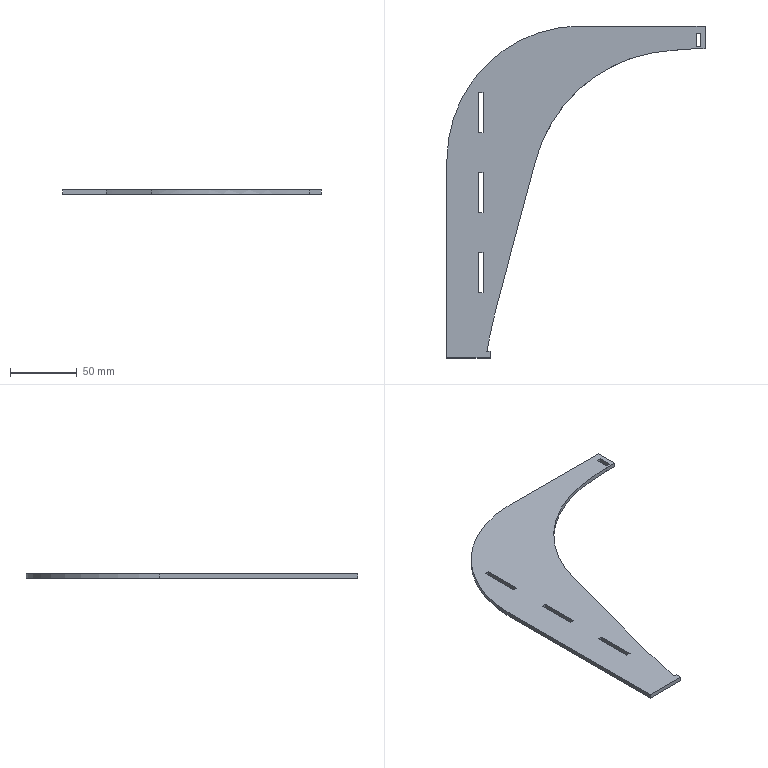Part | SolidWorks | features FlatPattern 1, SMBaseFlange 1, SheetMetal 1 | 1 solid | 31 faces | box 193.405 x 248.788 x 3.2 mm | volume 50560 mm3 | plane 26 | spline 3 | cylinder 2 | commonest cylinder face diameters 200 x1 887.053 x1
STEP:
#1=CARTESIAN_POINT('',(-170.654,-16.016,0.));
#2=VERTEX_POINT('',#1);
#3=CARTESIAN_POINT('',(-52.245,67.625,0.));
#4=VERTEX_POINT('',#3);
#5=CARTESIAN_POINT('',(-170.654,-16.016,0.));
#6=CARTESIAN_POINT('',(-168.965,-9.713,0.));
#7=CARTESIAN_POINT('',(-166.726,-3.585,0.));
#8=CARTESIAN_POINT('',(-161.155,8.306,0.));
#9=CARTESIAN_POINT('',(-157.878,13.952,0.));
#10=CARTESIAN_POINT('',(-150.345,24.639,0.));
#11=CARTESIAN_POINT('',(-146.124,29.625,0.));
#12=CARTESIAN_POINT('',(-139.114,36.565,0.));
#13=CARTESIAN_POINT('',(-135.476,39.865,0.));
#14=CARTESIAN_POINT('',(-130.997,43.416,0.));
#15=CARTESIAN_POINT('',(-129.027,44.874,0.));
#16=CARTESIAN_POINT('',(-127.703,45.832,0.));
#17=CARTESIAN_POINT('',(-127.037,46.303,0.));
#18=CARTESIAN_POINT('',(-120.965,50.494,0.));
#19=CARTESIAN_POINT('',(-115.278,53.719,0.));
#20=CARTESIAN_POINT('',(-103.335,59.164,0.));
#21=CARTESIAN_POINT('',(-97.175,61.342,0.));
#22=CARTESIAN_POINT('',(-89.232,63.383,0.));
#23=CARTESIAN_POINT('',(-86.84,63.941,0.));
#24=CARTESIAN_POINT('',(-84.034,64.499,0.));
#25=CARTESIAN_POINT('',(-82.627,64.754,0.));
#26=CARTESIAN_POINT('',(-82.023,64.858,0.));
#27=CARTESIAN_POINT('',(-81.62,64.926,0.));
#28=CARTESIAN_POINT('',(-81.417,64.96,0.));
#29=CARTESIAN_POINT('',(-80.419,65.124,0.));
#30=CARTESIAN_POINT('',(-79.214,65.308,0.));
#31=CARTESIAN_POINT('',(-77.793,65.502,0.));
#32=CARTESIAN_POINT('',(-77.079,65.593,0.));
#33=CARTESIAN_POINT('',(-76.721,65.637,0.));
#34=CARTESIAN_POINT('',(-76.542,65.659,0.));
#35=CARTESIAN_POINT('',(-76.452,65.67,0.));
#36=CARTESIAN_POINT('',(-76.407,65.676,0.));
#37=CARTESIAN_POINT('',(-76.388,65.678,0.));
#38=CARTESIAN_POINT('',(-76.375,65.679,0.));
#39=CARTESIAN_POINT('',(-76.368,65.68,0.));
#40=CARTESIAN_POINT('',(-75.713,65.759,0.));
#41=CARTESIAN_POINT('',(-74.62,65.88,0.));
#42=CARTESIAN_POINT('',(-73.139,66.029,0.));
#43=CARTESIAN_POINT('',(-72.346,66.106,0.));
#44=CARTESIAN_POINT('',(-71.937,66.145,0.));
#45=CARTESIAN_POINT('',(-71.729,66.164,0.));
#46=CARTESIAN_POINT('',(-71.625,66.174,0.));
#47=CARTESIAN_POINT('',(-71.572,66.179,0.));
#48=CARTESIAN_POINT('',(-71.55,66.181,0.));
#49=CARTESIAN_POINT('',(-71.535,66.182,0.));
#50=CARTESIAN_POINT('',(-71.526,66.183,0.));
#51=CARTESIAN_POINT('',(-65.156,66.776,0.));
#52=CARTESIAN_POINT('',(-58.732,67.256,0.));
#53=CARTESIAN_POINT('',(-52.245,67.625,0.));
#54=B_SPLINE_CURVE_WITH_KNOTS('',3,(#5,#6,#7,#8,#9,#10,#11,#12,#13,#14,#15,#16,#17,#18,#19,#20,#21,#22,#23,#24,#25,#26,#27,#28,#29,#30,#31,#32,#33,#34,#35,#36,#37,#38,#39,#40,#41,#42,#43,#44,#45,#46,#47,#48,#49,#50,#51,#52,#53),.UNSPECIFIED.,.F.,.F.,(4,2,2,2,1,1,2,2,2,2,1,1,1,2,2,1,1,1,1,1,1,1,2,2,1,1,1,1,1,1,1,2,2,4),(0.,0.125,0.25,0.375,0.4375,0.4688,0.4844,0.5,0.625,0.75,0.7813,0.7969,0.8047,0.8086,0.8125,0.8281,0.8359,0.8398,0.8418,0.8428,0.8433,0.8435,0.8436,0.8438,0.8594,0.8672,0.8711,0.873,0.874,0.8745,0.8748,0.8749,0.875,1.),.UNSPECIFIED.);
#55=EDGE_CURVE('',#2,#4,#54,.T.);
#56=ORIENTED_EDGE('',*,*,#55,.F.);
#57=CARTESIAN_POINT('',(-170.654,-16.016,-3.2));
#58=VERTEX_POINT('',#57);
#59=CARTESIAN_POINT('',(-170.654,-16.016,-3.2));
#60=DIRECTION('',(0.,0.,1.));
#61=VECTOR('',#60,1000.);
#62=LINE('',#59,#61);
#63=EDGE_CURVE('',#58,#2,#62,.T.);
#64=ORIENTED_EDGE('',*,*,#63,.F.);
#65=CARTESIAN_POINT('',(-52.245,67.625,-3.2));
#66=VERTEX_POINT('',#65);
#67=CARTESIAN_POINT('',(-170.654,-16.016,-3.2));
#68=CARTESIAN_POINT('',(-167.275,-3.408,-3.2));
#69=CARTESIAN_POINT('',(-161.645,8.608,-3.2));
#70=CARTESIAN_POINT('',(-146.578,29.983,-3.2));
#71=CARTESIAN_POINT('',(-137.134,39.334,-3.2));
#72=CARTESIAN_POINT('',(-120.976,50.486,-3.2));
#73=CARTESIAN_POINT('',(-115.261,53.727,-3.2));
#74=CARTESIAN_POINT('',(-103.352,59.157,-3.2));
#75=CARTESIAN_POINT('',(-97.158,61.346,-3.2));
#76=CARTESIAN_POINT('',(-87.652,63.789,-3.2));
#77=CARTESIAN_POINT('',(-84.447,64.463,-3.2));
#78=CARTESIAN_POINT('',(-79.602,65.258,-3.2));
#79=CARTESIAN_POINT('',(-77.981,65.487,-3.2));
#80=CARTESIAN_POINT('',(-74.744,65.875,-3.2));
#81=CARTESIAN_POINT('',(-73.129,66.034,-3.2));
#82=CARTESIAN_POINT('',(-68.301,66.483,-3.2));
#83=CARTESIAN_POINT('',(-65.1,66.748,-3.2));
#84=CARTESIAN_POINT('',(-58.675,67.229,-3.2));
#85=CARTESIAN_POINT('',(-55.46,67.442,-3.2));
#86=CARTESIAN_POINT('',(-52.245,67.625,-3.2));
#87=B_SPLINE_CURVE_WITH_KNOTS('',3,(#67,#68,#69,#70,#71,#72,#73,#74,#75,#76,#77,#78,#79,#80,#81,#82,#83,#84,#85,#86),.UNSPECIFIED.,.F.,.F.,(4,2,2,2,2,2,2,2,2,4),(0.,0.25,0.5,0.625,0.75,0.8125,0.8438,0.875,0.9375,1.),.UNSPECIFIED.);
#88=EDGE_CURVE('',#58,#66,#87,.T.);
#89=ORIENTED_EDGE('',*,*,#88,.T.);
#90=CARTESIAN_POINT('',(-52.245,67.625,-3.2));
#91=DIRECTION('',(0.,0.,1.));
#92=VECTOR('',#91,1000.);
#93=LINE('',#90,#92);
#94=EDGE_CURVE('',#66,#4,#93,.T.);
#95=ORIENTED_EDGE('',*,*,#94,.T.);
#96=EDGE_LOOP('',(#56,#64,#89,#95));
#97=FACE_OUTER_BOUND('',#96,.T.);
#98=CARTESIAN_POINT('',(-170.654,-16.016,-3.2));
#99=CARTESIAN_POINT('',(-170.654,-16.016,0.));
#100=CARTESIAN_POINT('',(-167.275,-3.408,-3.2));
#101=CARTESIAN_POINT('',(-167.275,-3.408,0.));
#102=CARTESIAN_POINT('',(-161.645,8.608,-3.2));
#103=CARTESIAN_POINT('',(-161.645,8.608,0.));
#104=CARTESIAN_POINT('',(-146.578,29.983,-3.2));
#105=CARTESIAN_POINT('',(-146.578,29.983,0.));
#106=CARTESIAN_POINT('',(-137.134,39.334,-3.2));
#107=CARTESIAN_POINT('',(-137.134,39.334,0.));
#108=CARTESIAN_POINT('',(-120.976,50.486,-3.2));
#109=CARTESIAN_POINT('',(-120.976,50.486,0.));
#110=CARTESIAN_POINT('',(-115.261,53.727,-3.2));
#111=CARTESIAN_POINT('',(-115.261,53.727,0.));
#112=CARTESIAN_POINT('',(-103.352,59.157,-3.2));
#113=CARTESIAN_POINT('',(-103.352,59.157,0.));
#114=CARTESIAN_POINT('',(-97.158,61.346,-3.2));
#115=CARTESIAN_POINT('',(-97.158,61.346,0.));
#116=CARTESIAN_POINT('',(-87.652,63.789,-3.2));
#117=CARTESIAN_POINT('',(-87.652,63.789,0.));
#118=CARTESIAN_POINT('',(-84.447,64.463,-3.2));
#119=CARTESIAN_POINT('',(-84.447,64.463,0.));
#120=CARTESIAN_POINT('',(-79.602,65.258,-3.2));
#121=CARTESIAN_POINT('',(-79.602,65.258,0.));
#122=CARTESIAN_POINT('',(-77.981,65.487,-3.2));
#123=CARTESIAN_POINT('',(-77.981,65.487,0.));
#124=CARTESIAN_POINT('',(-74.744,65.875,-3.2));
#125=CARTESIAN_POINT('',(-74.744,65.875,0.));
#126=CARTESIAN_POINT('',(-73.129,66.034,-3.2));
#127=CARTESIAN_POINT('',(-73.129,66.034,0.));
#128=CARTESIAN_POINT('',(-68.301,66.483,-3.2));
#129=CARTESIAN_POINT('',(-68.301,66.483,0.));
#130=CARTESIAN_POINT('',(-65.1,66.748,-3.2));
#131=CARTESIAN_POINT('',(-65.1,66.748,0.));
#132=CARTESIAN_POINT('',(-58.675,67.229,-3.2));
#133=CARTESIAN_POINT('',(-58.675,67.229,0.));
#134=CARTESIAN_POINT('',(-55.46,67.442,-3.2));
#135=CARTESIAN_POINT('',(-55.46,67.442,0.));
#136=CARTESIAN_POINT('',(-52.245,67.625,-3.2));
#137=CARTESIAN_POINT('',(-52.245,67.625,0.));
#138=B_SPLINE_SURFACE_WITH_KNOTS('',3,1,((#98,#99),(#100,#101),(#102,#103),(#104,#105),(#106,#107),(#108,#109),(#110,#111),(#112,#113),(#114,#115),(#116,#117),(#118,#119),(#120,#121),(#122,#123),(#124,#125),(#126,#127),(#128,#129),(#130,#131),(#132,#133),(#134,#135),(#136,#137)),.UNSPECIFIED.,.F.,.F.,.F.,(4,2,2,2,2,2,2,2,2,4),(2,2),(0.,0.25,0.5,0.625,0.75,0.8125,0.8438,0.875,0.9375,1.),(0.,1.),.UNSPECIFIED.);
#139=ADVANCED_FACE('',(#97),#138,.T.);
#140=CARTESIAN_POINT('',(-197.512,-116.241,0.));
#141=VERTEX_POINT('',#140);
#142=CARTESIAN_POINT('',(-170.654,-16.016,0.));
#143=DIRECTION('',(0.2588,0.9659,0.));
#144=VECTOR('',#143,1000.);
#145=LINE('',#142,#144);
#146=EDGE_CURVE('',#141,#2,#145,.T.);
#147=ORIENTED_EDGE('',*,*,#146,.F.);
#148=CARTESIAN_POINT('',(-197.512,-116.241,-3.2));
#149=VERTEX_POINT('',#148);
#150=CARTESIAN_POINT('',(-197.512,-116.241,-3.2));
#151=DIRECTION('',(0.,0.,1.));
#152=VECTOR('',#151,1000.);
#153=LINE('',#150,#152);
#154=EDGE_CURVE('',#149,#141,#153,.T.);
#155=ORIENTED_EDGE('',*,*,#154,.F.);
#156=CARTESIAN_POINT('',(-170.654,-16.016,-3.2));
#157=DIRECTION('',(0.2588,0.9659,0.));
#158=VECTOR('',#157,1000.);
#159=LINE('',#156,#158);
#160=EDGE_CURVE('',#149,#58,#159,.T.);
#161=ORIENTED_EDGE('',*,*,#160,.T.);
#162=ORIENTED_EDGE('',*,*,#63,.T.);
#163=EDGE_LOOP('',(#147,#155,#161,#162));
#164=FACE_OUTER_BOUND('',#163,.T.);
#165=CARTESIAN_POINT('',(-170.654,-16.016,-3.2));
#166=DIRECTION('',(0.9659,-0.2588,0.));
#167=DIRECTION('',(0.2588,0.9659,0.));
#168=AXIS2_PLACEMENT_3D('',#165,#166,#167);
#169=PLANE('',#168);
#170=ADVANCED_FACE('',(#164),#169,.T.);
#171=CARTESIAN_POINT('',(-204.762,-146.756,0.));
#172=VERTEX_POINT('',#171);
#173=CARTESIAN_POINT('',(230.108,-233.959,0.));
#174=DIRECTION('',(0.,0.,-1.));
#175=DIRECTION('',(-1.,0.,0.));
#176=AXIS2_PLACEMENT_3D('',#173,#174,#175);
#177=CIRCLE('',#176,443.526);
#178=EDGE_CURVE('',#172,#141,#177,.T.);
#179=ORIENTED_EDGE('',*,*,#178,.F.);
#180=CARTESIAN_POINT('',(-204.762,-146.756,-3.2));
#181=VERTEX_POINT('',#180);
#182=CARTESIAN_POINT('',(-204.762,-146.756,-3.2));
#183=DIRECTION('',(0.,0.,1.));
#184=VECTOR('',#183,1000.);
#185=LINE('',#182,#184);
#186=EDGE_CURVE('',#181,#172,#185,.T.);
#187=ORIENTED_EDGE('',*,*,#186,.F.);
#188=CARTESIAN_POINT('',(230.108,-233.959,-3.2));
#189=DIRECTION('',(0.,0.,-1.));
#190=DIRECTION('',(-1.,0.,0.));
#191=AXIS2_PLACEMENT_3D('',#188,#189,#190);
#192=CIRCLE('',#191,443.526);
#193=EDGE_CURVE('',#181,#149,#192,.T.);
#194=ORIENTED_EDGE('',*,*,#193,.T.);
#195=ORIENTED_EDGE('',*,*,#154,.T.);
#196=EDGE_LOOP('',(#179,#187,#194,#195));
#197=FACE_OUTER_BOUND('',#196,.T.);
#198=CARTESIAN_POINT('',(230.108,-233.959,-3.2));
#199=DIRECTION('',(0.,0.,1.));
#200=DIRECTION('',(1.,0.,0.));
#201=AXIS2_PLACEMENT_3D('',#198,#199,#200);
#202=CYLINDRICAL_SURFACE('',#201,443.526);
#203=ADVANCED_FACE('',(#197),#202,.F.);
#204=CARTESIAN_POINT('',(-207.067,-158.321,0.));
#205=VERTEX_POINT('',#204);
#206=CARTESIAN_POINT('',(-207.067,-158.321,0.));
#207=CARTESIAN_POINT('',(-206.479,-155.308,0.));
#208=CARTESIAN_POINT('',(-205.71,-151.453,0.));
#209=CARTESIAN_POINT('',(-204.762,-146.756,0.));
#210=B_SPLINE_CURVE_WITH_KNOTS('',3,(#206,#207,#208,#209),.UNSPECIFIED.,.F.,.F.,(4,4),(0.,1.),.UNSPECIFIED.);
#211=EDGE_CURVE('',#205,#172,#210,.T.);
#212=ORIENTED_EDGE('',*,*,#211,.F.);
#213=CARTESIAN_POINT('',(-207.067,-158.321,-3.2));
#214=VERTEX_POINT('',#213);
#215=CARTESIAN_POINT('',(-207.067,-158.321,-3.2));
#216=DIRECTION('',(0.,0.,1.));
#217=VECTOR('',#216,1000.);
#218=LINE('',#215,#217);
#219=EDGE_CURVE('',#214,#205,#218,.T.);
#220=ORIENTED_EDGE('',*,*,#219,.F.);
#221=CARTESIAN_POINT('',(-207.067,-158.321,-3.2));
#222=CARTESIAN_POINT('',(-206.57,-155.776,-3.2));
#223=CARTESIAN_POINT('',(-205.994,-152.886,-3.2));
#224=CARTESIAN_POINT('',(-205.529,-150.554,-3.2));
#225=CARTESIAN_POINT('',(-204.762,-146.756,-3.2));
#226=B_SPLINE_CURVE_WITH_KNOTS('',2,(#221,#222,#223,#224,#225),.UNSPECIFIED.,.F.,.F.,(3,2,3),(0.,0.5,1.),.UNSPECIFIED.);
#227=EDGE_CURVE('',#214,#181,#226,.T.);
#228=ORIENTED_EDGE('',*,*,#227,.T.);
#229=ORIENTED_EDGE('',*,*,#186,.T.);
#230=EDGE_LOOP('',(#212,#220,#228,#229));
#231=FACE_OUTER_BOUND('',#230,.T.);
#232=CARTESIAN_POINT('',(-207.067,-158.321,-3.2));
#233=CARTESIAN_POINT('',(-207.067,-158.321,0.));
#234=CARTESIAN_POINT('',(-206.57,-155.776,-3.2));
#235=CARTESIAN_POINT('',(-206.57,-155.776,0.));
#236=CARTESIAN_POINT('',(-205.994,-152.886,-3.2));
#237=CARTESIAN_POINT('',(-205.994,-152.886,0.));
#238=CARTESIAN_POINT('',(-205.529,-150.554,-3.2));
#239=CARTESIAN_POINT('',(-205.529,-150.554,0.));
#240=CARTESIAN_POINT('',(-204.762,-146.756,-3.2));
#241=CARTESIAN_POINT('',(-204.762,-146.756,0.));
#242=B_SPLINE_SURFACE_WITH_KNOTS('',2,1,((#232,#233),(#234,#235),(#236,#237),(#238,#239),(#240,#241)),.UNSPECIFIED.,.F.,.F.,.F.,(3,2,3),(2,2),(0.,0.5,1.),(0.,1.),.UNSPECIFIED.);
#243=ADVANCED_FACE('',(#231),#242,.T.);
#244=CARTESIAN_POINT('',(-207.184,-159.22,0.));
#245=VERTEX_POINT('',#244);
#246=CARTESIAN_POINT('',(-207.184,-159.22,0.));
#247=CARTESIAN_POINT('',(-207.159,-158.917,0.));
#248=CARTESIAN_POINT('',(-207.12,-158.617,0.));
#249=CARTESIAN_POINT('',(-207.067,-158.321,0.));
#250=B_SPLINE_CURVE_WITH_KNOTS('',3,(#246,#247,#248,#249),.UNSPECIFIED.,.F.,.F.,(4,4),(0.,1.),.UNSPECIFIED.);
#251=EDGE_CURVE('',#245,#205,#250,.T.);
#252=ORIENTED_EDGE('',*,*,#251,.F.);
#253=CARTESIAN_POINT('',(-207.184,-159.22,-3.2));
#254=VERTEX_POINT('',#253);
#255=CARTESIAN_POINT('',(-207.184,-159.22,-3.2));
#256=DIRECTION('',(0.,0.,1.));
#257=VECTOR('',#256,1000.);
#258=LINE('',#255,#257);
#259=EDGE_CURVE('',#254,#245,#258,.T.);
#260=ORIENTED_EDGE('',*,*,#259,.F.);
#261=CARTESIAN_POINT('',(-207.184,-159.22,-3.2));
#262=CARTESIAN_POINT('',(-207.172,-159.069,-3.2));
#263=CARTESIAN_POINT('',(-207.146,-158.766,-3.2));
#264=CARTESIAN_POINT('',(-207.094,-158.469,-3.2));
#265=CARTESIAN_POINT('',(-207.067,-158.321,-3.2));
#266=B_SPLINE_CURVE_WITH_KNOTS('',3,(#261,#262,#263,#264,#265),.UNSPECIFIED.,.F.,.F.,(4,1,4),(0.,0.5005,1.),.UNSPECIFIED.);
#267=EDGE_CURVE('',#254,#214,#266,.T.);
#268=ORIENTED_EDGE('',*,*,#267,.T.);
#269=ORIENTED_EDGE('',*,*,#219,.T.);
#270=EDGE_LOOP('',(#252,#260,#268,#269));
#271=FACE_OUTER_BOUND('',#270,.T.);
#272=CARTESIAN_POINT('',(-207.184,-159.22,-3.2));
#273=CARTESIAN_POINT('',(-207.184,-159.22,0.));
#274=CARTESIAN_POINT('',(-207.172,-159.069,-3.2));
#275=CARTESIAN_POINT('',(-207.172,-159.069,0.));
#276=CARTESIAN_POINT('',(-207.146,-158.766,-3.2));
#277=CARTESIAN_POINT('',(-207.146,-158.766,0.));
#278=CARTESIAN_POINT('',(-207.094,-158.469,-3.2));
#279=CARTESIAN_POINT('',(-207.094,-158.469,0.));
#280=CARTESIAN_POINT('',(-207.067,-158.321,-3.2));
#281=CARTESIAN_POINT('',(-207.067,-158.321,0.));
#282=B_SPLINE_SURFACE_WITH_KNOTS('',3,1,((#272,#273),(#274,#275),(#276,#277),(#278,#279),(#280,#281)),.UNSPECIFIED.,.F.,.F.,.F.,(4,1,4),(2,2),(0.,0.5005,1.),(0.,1.),.UNSPECIFIED.);
#283=ADVANCED_FACE('',(#271),#282,.T.);
#284=CARTESIAN_POINT('',(-204.879,-159.063,0.));
#285=VERTEX_POINT('',#284);
#286=CARTESIAN_POINT('',(-207.184,-159.22,0.));
#287=DIRECTION('',(-0.9977,-0.06788,0.));
#288=VECTOR('',#287,1000.);
#289=LINE('',#286,#288);
#290=EDGE_CURVE('',#285,#245,#289,.T.);
#291=ORIENTED_EDGE('',*,*,#290,.F.);
#292=CARTESIAN_POINT('',(-204.879,-159.063,-3.2));
#293=VERTEX_POINT('',#292);
#294=CARTESIAN_POINT('',(-204.879,-159.063,-3.2));
#295=DIRECTION('',(0.,0.,1.));
#296=VECTOR('',#295,1000.);
#297=LINE('',#294,#296);
#298=EDGE_CURVE('',#293,#285,#297,.T.);
#299=ORIENTED_EDGE('',*,*,#298,.F.);
#300=CARTESIAN_POINT('',(-207.184,-159.22,-3.2));
#301=DIRECTION('',(-0.9977,-0.06788,0.));
#302=VECTOR('',#301,1000.);
#303=LINE('',#300,#302);
#304=EDGE_CURVE('',#293,#254,#303,.T.);
#305=ORIENTED_EDGE('',*,*,#304,.T.);
#306=ORIENTED_EDGE('',*,*,#259,.T.);
#307=EDGE_LOOP('',(#291,#299,#305,#306));
#308=FACE_OUTER_BOUND('',#307,.T.);
#309=CARTESIAN_POINT('',(-207.184,-159.22,-3.2));
#310=DIRECTION('',(-0.06788,0.9977,0.));
#311=DIRECTION('',(-0.9977,-0.06788,0.));
#312=AXIS2_PLACEMENT_3D('',#309,#310,#311);
#313=PLANE('',#312);
#314=ADVANCED_FACE('',(#308),#313,.T.);
#315=CARTESIAN_POINT('',(-204.879,-164.063,0.));
#316=VERTEX_POINT('',#315);
#317=CARTESIAN_POINT('',(-204.879,-164.063,0.));
#318=DIRECTION('',(0.,1.,0.));
#319=VECTOR('',#318,1000.);
#320=LINE('',#317,#319);
#321=EDGE_CURVE('',#316,#285,#320,.T.);
#322=ORIENTED_EDGE('',*,*,#321,.F.);
#323=CARTESIAN_POINT('',(-204.879,-164.063,-3.2));
#324=VERTEX_POINT('',#323);
#325=CARTESIAN_POINT('',(-204.879,-164.063,-3.2));
#326=DIRECTION('',(0.,0.,1.));
#327=VECTOR('',#326,1000.);
#328=LINE('',#325,#327);
#329=EDGE_CURVE('',#324,#316,#328,.T.);
#330=ORIENTED_EDGE('',*,*,#329,.F.);
#331=CARTESIAN_POINT('',(-204.879,-164.063,-3.2));
#332=DIRECTION('',(0.,1.,0.));
#333=VECTOR('',#332,1000.);
#334=LINE('',#331,#333);
#335=EDGE_CURVE('',#324,#293,#334,.T.);
#336=ORIENTED_EDGE('',*,*,#335,.T.);
#337=ORIENTED_EDGE('',*,*,#298,.T.);
#338=EDGE_LOOP('',(#322,#330,#336,#337));
#339=FACE_OUTER_BOUND('',#338,.T.);
#340=CARTESIAN_POINT('',(-204.879,-164.063,-3.2));
#341=DIRECTION('',(1.,0.,0.));
#342=DIRECTION('',(0.,1.,0.));
#343=AXIS2_PLACEMENT_3D('',#340,#341,#342);
#344=PLANE('',#343);
#345=ADVANCED_FACE('',(#339),#344,.T.);
#346=CARTESIAN_POINT('',(-237.15,-164.063,0.));
#347=VERTEX_POINT('',#346);
#348=CARTESIAN_POINT('',(-237.15,-164.063,0.));
#349=DIRECTION('',(1.,0.,0.));
#350=VECTOR('',#349,1000.);
#351=LINE('',#348,#350);
#352=EDGE_CURVE('',#347,#316,#351,.T.);
#353=ORIENTED_EDGE('',*,*,#352,.F.);
#354=CARTESIAN_POINT('',(-237.15,-164.063,-3.2));
#355=VERTEX_POINT('',#354);
#356=CARTESIAN_POINT('',(-237.15,-164.063,-3.2));
#357=DIRECTION('',(0.,0.,1.));
#358=VECTOR('',#357,1000.);
#359=LINE('',#356,#358);
#360=EDGE_CURVE('',#355,#347,#359,.T.);
#361=ORIENTED_EDGE('',*,*,#360,.F.);
#362=CARTESIAN_POINT('',(-237.15,-164.063,-3.2));
#363=DIRECTION('',(1.,0.,0.));
#364=VECTOR('',#363,1000.);
#365=LINE('',#362,#364);
#366=EDGE_CURVE('',#355,#324,#365,.T.);
#367=ORIENTED_EDGE('',*,*,#366,.T.);
#368=ORIENTED_EDGE('',*,*,#329,.T.);
#369=EDGE_LOOP('',(#353,#361,#367,#368));
#370=FACE_OUTER_BOUND('',#369,.T.);
#371=CARTESIAN_POINT('',(-237.15,-164.063,-3.2));
#372=DIRECTION('',(0.,-1.,0.));
#373=DIRECTION('',(0.,0.,-1.));
#374=AXIS2_PLACEMENT_3D('',#371,#372,#373);
#375=PLANE('',#374);
#376=ADVANCED_FACE('',(#370),#375,.T.);
#377=CARTESIAN_POINT('',(-237.15,-15.276,0.));
#378=VERTEX_POINT('',#377);
#379=CARTESIAN_POINT('',(-237.15,-15.276,0.));
#380=DIRECTION('',(0.,-1.,0.));
#381=VECTOR('',#380,1000.);
#382=LINE('',#379,#381);
#383=EDGE_CURVE('',#378,#347,#382,.T.);
#384=ORIENTED_EDGE('',*,*,#383,.F.);
#385=CARTESIAN_POINT('',(-237.15,-15.276,-3.2));
#386=VERTEX_POINT('',#385);
#387=CARTESIAN_POINT('',(-237.15,-15.276,-3.2));
#388=DIRECTION('',(0.,0.,1.));
#389=VECTOR('',#388,1000.);
#390=LINE('',#387,#389);
#391=EDGE_CURVE('',#386,#378,#390,.T.);
#392=ORIENTED_EDGE('',*,*,#391,.F.);
#393=CARTESIAN_POINT('',(-237.15,-15.276,-3.2));
#394=DIRECTION('',(0.,-1.,0.));
#395=VECTOR('',#394,1000.);
#396=LINE('',#393,#395);
#397=EDGE_CURVE('',#386,#355,#396,.T.);
#398=ORIENTED_EDGE('',*,*,#397,.T.);
#399=ORIENTED_EDGE('',*,*,#360,.T.);
#400=EDGE_LOOP('',(#384,#392,#398,#399));
#401=FACE_OUTER_BOUND('',#400,.T.);
#402=CARTESIAN_POINT('',(-237.15,-15.276,-3.2));
#403=DIRECTION('',(-1.,0.,0.));
#404=DIRECTION('',(0.,-1.,0.));
#405=AXIS2_PLACEMENT_3D('',#402,#403,#404);
#406=PLANE('',#405);
#407=ADVANCED_FACE('',(#401),#406,.T.);
#408=CARTESIAN_POINT('',(-137.15,84.724,0.));
#409=VERTEX_POINT('',#408);
#410=CARTESIAN_POINT('',(-137.15,-15.276,0.));
#411=DIRECTION('',(0.,0.,1.));
#412=DIRECTION('',(-1.,0.,0.));
#413=AXIS2_PLACEMENT_3D('',#410,#411,#412);
#414=CIRCLE('',#413,100.);
#415=EDGE_CURVE('',#409,#378,#414,.T.);
#416=ORIENTED_EDGE('',*,*,#415,.F.);
#417=CARTESIAN_POINT('',(-137.15,84.724,-3.2));
#418=VERTEX_POINT('',#417);
#419=CARTESIAN_POINT('',(-137.15,84.724,-3.2));
#420=DIRECTION('',(0.,0.,1.));
#421=VECTOR('',#420,1000.);
#422=LINE('',#419,#421);
#423=EDGE_CURVE('',#418,#409,#422,.T.);
#424=ORIENTED_EDGE('',*,*,#423,.F.);
#425=CARTESIAN_POINT('',(-137.15,-15.276,-3.2));
#426=DIRECTION('',(0.,0.,1.));
#427=DIRECTION('',(-1.,0.,0.));
#428=AXIS2_PLACEMENT_3D('',#425,#426,#427);
#429=CIRCLE('',#428,100.);
#430=EDGE_CURVE('',#418,#386,#429,.T.);
#431=ORIENTED_EDGE('',*,*,#430,.T.);
#432=ORIENTED_EDGE('',*,*,#391,.T.);
#433=EDGE_LOOP('',(#416,#424,#431,#432));
#434=FACE_OUTER_BOUND('',#433,.T.);
#435=CARTESIAN_POINT('',(-137.15,-15.276,-3.2));
#436=DIRECTION('',(0.,0.,1.));
#437=DIRECTION('',(1.,0.,0.));
#438=AXIS2_PLACEMENT_3D('',#435,#436,#437);
#439=CYLINDRICAL_SURFACE('',#438,100.);
#440=ADVANCED_FACE('',(#434),#439,.T.);
#441=CARTESIAN_POINT('',(-43.745,84.724,0.));
#442=VERTEX_POINT('',#441);
#443=CARTESIAN_POINT('',(-43.745,84.724,0.));
#444=DIRECTION('',(-1.,0.,0.));
#445=VECTOR('',#444,1000.);
#446=LINE('',#443,#445);
#447=EDGE_CURVE('',#442,#409,#446,.T.);
#448=ORIENTED_EDGE('',*,*,#447,.F.);
#449=CARTESIAN_POINT('',(-43.745,84.724,-3.2));
#450=VERTEX_POINT('',#449);
#451=CARTESIAN_POINT('',(-43.745,84.724,-3.2));
#452=DIRECTION('',(0.,0.,1.));
#453=VECTOR('',#452,1000.);
#454=LINE('',#451,#453);
#455=EDGE_CURVE('',#450,#442,#454,.T.);
#456=ORIENTED_EDGE('',*,*,#455,.F.);
#457=CARTESIAN_POINT('',(-43.745,84.724,-3.2));
#458=DIRECTION('',(-1.,0.,0.));
#459=VECTOR('',#458,1000.);
#460=LINE('',#457,#459);
#461=EDGE_CURVE('',#450,#418,#460,.T.);
#462=ORIENTED_EDGE('',*,*,#461,.T.);
#463=ORIENTED_EDGE('',*,*,#423,.T.);
#464=EDGE_LOOP('',(#448,#456,#462,#463));
#465=FACE_OUTER_BOUND('',#464,.T.);
#466=CARTESIAN_POINT('',(-43.745,84.724,-3.2));
#467=DIRECTION('',(0.,1.,0.));
#468=DIRECTION('',(-1.,0.,0.));
#469=AXIS2_PLACEMENT_3D('',#466,#467,#468);
#470=PLANE('',#469);
#471=ADVANCED_FACE('',(#465),#470,.T.);
#472=CARTESIAN_POINT('',(-43.745,67.625,0.));
#473=VERTEX_POINT('',#472);
#474=CARTESIAN_POINT('',(-43.745,84.724,0.));
#475=DIRECTION('',(0.,1.,0.));
#476=VECTOR('',#475,1000.);
#477=LINE('',#474,#476);
#478=EDGE_CURVE('',#473,#442,#477,.T.);
#479=ORIENTED_EDGE('',*,*,#478,.F.);
#480=CARTESIAN_POINT('',(-43.745,67.625,-3.2));
#481=VERTEX_POINT('',#480);
#482=CARTESIAN_POINT('',(-43.745,67.625,-3.2));
#483=DIRECTION('',(0.,0.,1.));
#484=VECTOR('',#483,1000.);
#485=LINE('',#482,#484);
#486=EDGE_CURVE('',#481,#473,#485,.T.);
#487=ORIENTED_EDGE('',*,*,#486,.F.);
#488=CARTESIAN_POINT('',(-43.745,84.724,-3.2));
#489=DIRECTION('',(0.,1.,0.));
#490=VECTOR('',#489,1000.);
#491=LINE('',#488,#490);
#492=EDGE_CURVE('',#481,#450,#491,.T.);
#493=ORIENTED_EDGE('',*,*,#492,.T.);
#494=ORIENTED_EDGE('',*,*,#455,.T.);
#495=EDGE_LOOP('',(#479,#487,#493,#494));
#496=FACE_OUTER_BOUND('',#495,.T.);
#497=CARTESIAN_POINT('',(-43.745,84.724,-3.2));
#498=DIRECTION('',(1.,0.,0.));
#499=DIRECTION('',(0.,0.,-1.));
#500=AXIS2_PLACEMENT_3D('',#497,#498,#499);
#501=PLANE('',#500);
#502=ADVANCED_FACE('',(#496),#501,.T.);
#503=CARTESIAN_POINT('',(-43.745,67.625,0.));
#504=DIRECTION('',(1.,0.,0.));
#505=VECTOR('',#504,1000.);
#506=LINE('',#503,#505);
#507=EDGE_CURVE('',#4,#473,#506,.T.);
#508=ORIENTED_EDGE('',*,*,#507,.F.);
#509=ORIENTED_EDGE('',*,*,#94,.F.);
#510=CARTESIAN_POINT('',(-43.745,67.625,-3.2));
#511=DIRECTION('',(1.,0.,0.));
#512=VECTOR('',#511,1000.);
#513=LINE('',#510,#512);
#514=EDGE_CURVE('',#66,#481,#513,.T.);
#515=ORIENTED_EDGE('',*,*,#514,.T.);
#516=ORIENTED_EDGE('',*,*,#486,.T.);
#517=EDGE_LOOP('',(#508,#509,#515,#516));
#518=FACE_OUTER_BOUND('',#517,.T.);
#519=CARTESIAN_POINT('',(-43.745,67.625,-3.2));
#520=DIRECTION('',(0.,-1.,0.));
#521=DIRECTION('',(0.,0.,-1.));
#522=AXIS2_PLACEMENT_3D('',#519,#520,#521);
#523=PLANE('',#522);
#524=ADVANCED_FACE('',(#518),#523,.T.);
#525=CARTESIAN_POINT('',(-213.292,-85.276,-3.2));
#526=VERTEX_POINT('',#525);
#527=CARTESIAN_POINT('',(-213.292,-115.276,-3.2));
#528=VERTEX_POINT('',#527);
#529=CARTESIAN_POINT('',(-213.292,-85.276,-3.2));
#530=DIRECTION('',(0.,-1.,0.));
#531=VECTOR('',#530,1000.);
#532=LINE('',#529,#531);
#533=EDGE_CURVE('',#526,#528,#532,.T.);
#534=ORIENTED_EDGE('',*,*,#533,.T.);
#535=CARTESIAN_POINT('',(-210.092,-115.276,-3.2));
#536=VERTEX_POINT('',#535);
#537=CARTESIAN_POINT('',(-213.292,-115.276,-3.2));
#538=DIRECTION('',(1.,0.,0.));
#539=VECTOR('',#538,1000.);
#540=LINE('',#537,#539);
#541=EDGE_CURVE('',#528,#536,#540,.T.);
#542=ORIENTED_EDGE('',*,*,#541,.T.);
#543=CARTESIAN_POINT('',(-210.092,-85.276,-3.2));
#544=VERTEX_POINT('',#543);
#545=CARTESIAN_POINT('',(-210.092,-85.276,-3.2));
#546=DIRECTION('',(0.,1.,0.));
#547=VECTOR('',#546,1000.);
#548=LINE('',#545,#547);
#549=EDGE_CURVE('',#536,#544,#548,.T.);
#550=ORIENTED_EDGE('',*,*,#549,.T.);
#551=CARTESIAN_POINT('',(-213.292,-85.276,-3.2));
#552=DIRECTION('',(-1.,0.,0.));
#553=VECTOR('',#552,1000.);
#554=LINE('',#551,#553);
#555=EDGE_CURVE('',#544,#526,#554,.T.);
#556=ORIENTED_EDGE('',*,*,#555,.T.);
#557=EDGE_LOOP('',(#534,#542,#550,#556));
#558=FACE_BOUND('',#557,.T.);
#559=CARTESIAN_POINT('',(-213.292,-25.276,-3.2));
#560=VERTEX_POINT('',#559);
#561=CARTESIAN_POINT('',(-213.292,-55.276,-3.2));
#562=VERTEX_POINT('',#561);
#563=CARTESIAN_POINT('',(-213.292,-25.276,-3.2));
#564=DIRECTION('',(0.,-1.,0.));
#565=VECTOR('',#564,1000.);
#566=LINE('',#563,#565);
#567=EDGE_CURVE('',#560,#562,#566,.T.);
#568=ORIENTED_EDGE('',*,*,#567,.T.);
#569=CARTESIAN_POINT('',(-210.092,-55.276,-3.2));
#570=VERTEX_POINT('',#569);
#571=CARTESIAN_POINT('',(-213.292,-55.276,-3.2));
#572=DIRECTION('',(1.,0.,0.));
#573=VECTOR('',#572,1000.);
#574=LINE('',#571,#573);
#575=EDGE_CURVE('',#562,#570,#574,.T.);
#576=ORIENTED_EDGE('',*,*,#575,.T.);
#577=CARTESIAN_POINT('',(-210.092,-25.276,-3.2));
#578=VERTEX_POINT('',#577);
#579=CARTESIAN_POINT('',(-210.092,-25.276,-3.2));
#580=DIRECTION('',(0.,1.,0.));
#581=VECTOR('',#580,1000.);
#582=LINE('',#579,#581);
#583=EDGE_CURVE('',#570,#578,#582,.T.);
#584=ORIENTED_EDGE('',*,*,#583,.T.);
#585=CARTESIAN_POINT('',(-213.292,-25.276,-3.2));
#586=DIRECTION('',(-1.,0.,0.));
#587=VECTOR('',#586,1000.);
#588=LINE('',#585,#587);
#589=EDGE_CURVE('',#578,#560,#588,.T.);
#590=ORIENTED_EDGE('',*,*,#589,.T.);
#591=EDGE_LOOP('',(#568,#576,#584,#590));
#592=FACE_BOUND('',#591,.T.);
#593=CARTESIAN_POINT('',(-213.292,34.724,-3.2));
#594=VERTEX_POINT('',#593);
#595=CARTESIAN_POINT('',(-213.292,4.724,-3.2));
#596=VERTEX_POINT('',#595);
#597=CARTESIAN_POINT('',(-213.292,34.724,-3.2));
#598=DIRECTION('',(0.,-1.,0.));
#599=VECTOR('',#598,1000.);
#600=LINE('',#597,#599);
#601=EDGE_CURVE('',#594,#596,#600,.T.);
#602=ORIENTED_EDGE('',*,*,#601,.T.);
#603=CARTESIAN_POINT('',(-210.092,4.724,-3.2));
#604=VERTEX_POINT('',#603);
#605=CARTESIAN_POINT('',(-213.292,4.724,-3.2));
#606=DIRECTION('',(1.,0.,0.));
#607=VECTOR('',#606,1000.);
#608=LINE('',#605,#607);
#609=EDGE_CURVE('',#596,#604,#608,.T.);
#610=ORIENTED_EDGE('',*,*,#609,.T.);
#611=CARTESIAN_POINT('',(-210.092,34.724,-3.2));
#612=VERTEX_POINT('',#611);
#613=CARTESIAN_POINT('',(-210.092,34.724,-3.2));
#614=DIRECTION('',(0.,1.,0.));
#615=VECTOR('',#614,1000.);
#616=LINE('',#613,#615);
#617=EDGE_CURVE('',#604,#612,#616,.T.);
#618=ORIENTED_EDGE('',*,*,#617,.T.);
#619=CARTESIAN_POINT('',(-213.292,34.724,-3.2));
#620=DIRECTION('',(-1.,0.,0.));
#621=VECTOR('',#620,1000.);
#622=LINE('',#619,#621);
#623=EDGE_CURVE('',#612,#594,#622,.T.);
#624=ORIENTED_EDGE('',*,*,#623,.T.);
#625=EDGE_LOOP('',(#602,#610,#618,#624));
#626=FACE_BOUND('',#625,.T.);
#627=CARTESIAN_POINT('',(-50.35,79.224,-3.2));
#628=VERTEX_POINT('',#627);
#629=CARTESIAN_POINT('',(-50.35,69.224,-3.2));
#630=VERTEX_POINT('',#629);
#631=CARTESIAN_POINT('',(-50.35,79.224,-3.2));
#632=DIRECTION('',(0.,-1.,0.));
#633=VECTOR('',#632,1000.);
#634=LINE('',#631,#633);
#635=EDGE_CURVE('',#628,#630,#634,.T.);
#636=ORIENTED_EDGE('',*,*,#635,.T.);
#637=CARTESIAN_POINT('',(-47.15,69.224,-3.2));
#638=VERTEX_POINT('',#637);
#639=CARTESIAN_POINT('',(-50.35,69.224,-3.2));
#640=DIRECTION('',(1.,0.,0.));
#641=VECTOR('',#640,1000.);
#642=LINE('',#639,#641);
#643=EDGE_CURVE('',#630,#638,#642,.T.);
#644=ORIENTED_EDGE('',*,*,#643,.T.);
#645=CARTESIAN_POINT('',(-47.15,79.224,-3.2));
#646=VERTEX_POINT('',#645);
#647=CARTESIAN_POINT('',(-47.15,79.224,-3.2));
#648=DIRECTION('',(0.,1.,0.));
#649=VECTOR('',#648,1000.);
#650=LINE('',#647,#649);
#651=EDGE_CURVE('',#638,#646,#650,.T.);
#652=ORIENTED_EDGE('',*,*,#651,.T.);
#653=CARTESIAN_POINT('',(-50.35,79.224,-3.2));
#654=DIRECTION('',(-1.,0.,0.));
#655=VECTOR('',#654,1000.);
#656=LINE('',#653,#655);
#657=EDGE_CURVE('',#646,#628,#656,.T.);
#658=ORIENTED_EDGE('',*,*,#657,.T.);
#659=EDGE_LOOP('',(#636,#644,#652,#658));
#660=FACE_BOUND('',#659,.T.);
#661=ORIENTED_EDGE('',*,*,#88,.F.);
#662=ORIENTED_EDGE('',*,*,#160,.F.);
#663=ORIENTED_EDGE('',*,*,#193,.F.);
#664=ORIENTED_EDGE('',*,*,#227,.F.);
#665=ORIENTED_EDGE('',*,*,#267,.F.);
#666=ORIENTED_EDGE('',*,*,#304,.F.);
#667=ORIENTED_EDGE('',*,*,#335,.F.);
#668=ORIENTED_EDGE('',*,*,#366,.F.);
#669=ORIENTED_EDGE('',*,*,#397,.F.);
#670=ORIENTED_EDGE('',*,*,#430,.F.);
#671=ORIENTED_EDGE('',*,*,#461,.F.);
#672=ORIENTED_EDGE('',*,*,#492,.F.);
#673=ORIENTED_EDGE('',*,*,#514,.F.);
#674=EDGE_LOOP('',(#661,#662,#663,#664,#665,#666,#667,#668,#669,#670,#671,#672,#673));
#675=FACE_OUTER_BOUND('',#674,.T.);
#676=CARTESIAN_POINT('',(-126.362,46.768,-3.2));
#677=DIRECTION('',(0.,0.,-1.));
#678=DIRECTION('',(-1.,0.,0.));
#679=AXIS2_PLACEMENT_3D('',#676,#677,#678);
#680=PLANE('',#679);
#681=ADVANCED_FACE('',(#558,#592,#626,#660,#675),#680,.T.);
#682=CARTESIAN_POINT('',(-213.292,-115.276,0.));
#683=VERTEX_POINT('',#682);
#684=CARTESIAN_POINT('',(-210.092,-115.276,0.));
#685=VERTEX_POINT('',#684);
#686=CARTESIAN_POINT('',(-213.292,-115.276,0.));
#687=DIRECTION('',(1.,0.,0.));
#688=VECTOR('',#687,1000.);
#689=LINE('',#686,#688);
#690=EDGE_CURVE('',#683,#685,#689,.T.);
#691=ORIENTED_EDGE('',*,*,#690,.F.);
#692=CARTESIAN_POINT('',(-213.292,-85.276,0.));
#693=VERTEX_POINT('',#692);
#694=CARTESIAN_POINT('',(-213.292,-85.276,0.));
#695=DIRECTION('',(0.,-1.,0.));
#696=VECTOR('',#695,1000.);
#697=LINE('',#694,#696);
#698=EDGE_CURVE('',#693,#683,#697,.T.);
#699=ORIENTED_EDGE('',*,*,#698,.F.);
#700=CARTESIAN_POINT('',(-210.092,-85.276,0.));
#701=VERTEX_POINT('',#700);
#702=CARTESIAN_POINT('',(-213.292,-85.276,0.));
#703=DIRECTION('',(-1.,0.,0.));
#704=VECTOR('',#703,1000.);
#705=LINE('',#702,#704);
#706=EDGE_CURVE('',#701,#693,#705,.T.);
#707=ORIENTED_EDGE('',*,*,#706,.F.);
#708=CARTESIAN_POINT('',(-210.092,-85.276,0.));
#709=DIRECTION('',(0.,1.,0.));
#710=VECTOR('',#709,1000.);
#711=LINE('',#708,#710);
#712=EDGE_CURVE('',#685,#701,#711,.T.);
#713=ORIENTED_EDGE('',*,*,#712,.F.);
#714=EDGE_LOOP('',(#691,#699,#707,#713));
#715=FACE_BOUND('',#714,.T.);
#716=CARTESIAN_POINT('',(-213.292,-55.276,0.));
#717=VERTEX_POINT('',#716);
#718=CARTESIAN_POINT('',(-210.092,-55.276,0.));
#719=VERTEX_POINT('',#718);
#720=CARTESIAN_POINT('',(-213.292,-55.276,0.));
#721=DIRECTION('',(1.,0.,0.));
#722=VECTOR('',#721,1000.);
#723=LINE('',#720,#722);
#724=EDGE_CURVE('',#717,#719,#723,.T.);
#725=ORIENTED_EDGE('',*,*,#724,.F.);
#726=CARTESIAN_POINT('',(-213.292,-25.276,0.));
#727=VERTEX_POINT('',#726);
#728=CARTESIAN_POINT('',(-213.292,-25.276,0.));
#729=DIRECTION('',(0.,-1.,0.));
#730=VECTOR('',#729,1000.);
#731=LINE('',#728,#730);
#732=EDGE_CURVE('',#727,#717,#731,.T.);
#733=ORIENTED_EDGE('',*,*,#732,.F.);
#734=CARTESIAN_POINT('',(-210.092,-25.276,0.));
#735=VERTEX_POINT('',#734);
#736=CARTESIAN_POINT('',(-213.292,-25.276,0.));
#737=DIRECTION('',(-1.,0.,0.));
#738=VECTOR('',#737,1000.);
#739=LINE('',#736,#738);
#740=EDGE_CURVE('',#735,#727,#739,.T.);
#741=ORIENTED_EDGE('',*,*,#740,.F.);
#742=CARTESIAN_POINT('',(-210.092,-25.276,0.));
#743=DIRECTION('',(0.,1.,0.));
#744=VECTOR('',#743,1000.);
#745=LINE('',#742,#744);
#746=EDGE_CURVE('',#719,#735,#745,.T.);
#747=ORIENTED_EDGE('',*,*,#746,.F.);
#748=EDGE_LOOP('',(#725,#733,#741,#747));
#749=FACE_BOUND('',#748,.T.);
#750=CARTESIAN_POINT('',(-213.292,4.724,0.));
#751=VERTEX_POINT('',#750);
#752=CARTESIAN_POINT('',(-210.092,4.724,0.));
#753=VERTEX_POINT('',#752);
#754=CARTESIAN_POINT('',(-213.292,4.724,0.));
#755=DIRECTION('',(1.,0.,0.));
#756=VECTOR('',#755,1000.);
#757=LINE('',#754,#756);
#758=EDGE_CURVE('',#751,#753,#757,.T.);
#759=ORIENTED_EDGE('',*,*,#758,.F.);
#760=CARTESIAN_POINT('',(-213.292,34.724,0.));
#761=VERTEX_POINT('',#760);
#762=CARTESIAN_POINT('',(-213.292,34.724,0.));
#763=DIRECTION('',(0.,-1.,0.));
#764=VECTOR('',#763,1000.);
#765=LINE('',#762,#764);
#766=EDGE_CURVE('',#761,#751,#765,.T.);
#767=ORIENTED_EDGE('',*,*,#766,.F.);
#768=CARTESIAN_POINT('',(-210.092,34.724,0.));
#769=VERTEX_POINT('',#768);
#770=CARTESIAN_POINT('',(-213.292,34.724,0.));
#771=DIRECTION('',(-1.,0.,0.));
#772=VECTOR('',#771,1000.);
#773=LINE('',#770,#772);
#774=EDGE_CURVE('',#769,#761,#773,.T.);
#775=ORIENTED_EDGE('',*,*,#774,.F.);
#776=CARTESIAN_POINT('',(-210.092,34.724,0.));
#777=DIRECTION('',(0.,1.,0.));
#778=VECTOR('',#777,1000.);
#779=LINE('',#776,#778);
#780=EDGE_CURVE('',#753,#769,#779,.T.);
#781=ORIENTED_EDGE('',*,*,#780,.F.);
#782=EDGE_LOOP('',(#759,#767,#775,#781));
#783=FACE_BOUND('',#782,.T.);
#784=CARTESIAN_POINT('',(-50.35,69.224,0.));
#785=VERTEX_POINT('',#784);
#786=CARTESIAN_POINT('',(-47.15,69.224,0.));
#787=VERTEX_POINT('',#786);
#788=CARTESIAN_POINT('',(-50.35,69.224,0.));
#789=DIRECTION('',(1.,0.,0.));
#790=VECTOR('',#789,1000.);
#791=LINE('',#788,#790);
#792=EDGE_CURVE('',#785,#787,#791,.T.);
#793=ORIENTED_EDGE('',*,*,#792,.F.);
#794=CARTESIAN_POINT('',(-50.35,79.224,0.));
#795=VERTEX_POINT('',#794);
#796=CARTESIAN_POINT('',(-50.35,79.224,0.));
#797=DIRECTION('',(0.,-1.,0.));
#798=VECTOR('',#797,1000.);
#799=LINE('',#796,#798);
#800=EDGE_CURVE('',#795,#785,#799,.T.);
#801=ORIENTED_EDGE('',*,*,#800,.F.);
#802=CARTESIAN_POINT('',(-47.15,79.224,0.));
#803=VERTEX_POINT('',#802);
#804=CARTESIAN_POINT('',(-50.35,79.224,0.));
#805=DIRECTION('',(-1.,0.,0.));
#806=VECTOR('',#805,1000.);
#807=LINE('',#804,#806);
#808=EDGE_CURVE('',#803,#795,#807,.T.);
#809=ORIENTED_EDGE('',*,*,#808,.F.);
#810=CARTESIAN_POINT('',(-47.15,79.224,0.));
#811=DIRECTION('',(0.,1.,0.));
#812=VECTOR('',#811,1000.);
#813=LINE('',#810,#812);
#814=EDGE_CURVE('',#787,#803,#813,.T.);
#815=ORIENTED_EDGE('',*,*,#814,.F.);
#816=EDGE_LOOP('',(#793,#801,#809,#815));
#817=FACE_BOUND('',#816,.T.);
#818=ORIENTED_EDGE('',*,*,#55,.T.);
#819=ORIENTED_EDGE('',*,*,#507,.T.);
#820=ORIENTED_EDGE('',*,*,#478,.T.);
#821=ORIENTED_EDGE('',*,*,#447,.T.);
#822=ORIENTED_EDGE('',*,*,#415,.T.);
#823=ORIENTED_EDGE('',*,*,#383,.T.);
#824=ORIENTED_EDGE('',*,*,#352,.T.);
#825=ORIENTED_EDGE('',*,*,#321,.T.);
#826=ORIENTED_EDGE('',*,*,#290,.T.);
#827=ORIENTED_EDGE('',*,*,#251,.T.);
#828=ORIENTED_EDGE('',*,*,#211,.T.);
#829=ORIENTED_EDGE('',*,*,#178,.T.);
#830=ORIENTED_EDGE('',*,*,#146,.T.);
#831=EDGE_LOOP('',(#818,#819,#820,#821,#822,#823,#824,#825,#826,#827,#828,#829,#830));
#832=FACE_OUTER_BOUND('',#831,.T.);
#833=CARTESIAN_POINT('',(-126.362,46.768,0.));
#834=DIRECTION('',(0.,0.,-1.));
#835=DIRECTION('',(-1.,0.,0.));
#836=AXIS2_PLACEMENT_3D('',#833,#834,#835);
#837=PLANE('',#836);
#838=ADVANCED_FACE('',(#715,#749,#783,#817,#832),#837,.F.);
#839=ORIENTED_EDGE('',*,*,#800,.T.);
#840=CARTESIAN_POINT('',(-50.35,69.224,-3.2));
#841=DIRECTION('',(0.,0.,1.));
#842=VECTOR('',#841,1000.);
#843=LINE('',#840,#842);
#844=EDGE_CURVE('',#630,#785,#843,.T.);
#845=ORIENTED_EDGE('',*,*,#844,.F.);
#846=ORIENTED_EDGE('',*,*,#635,.F.);
#847=CARTESIAN_POINT('',(-50.35,79.224,-3.2));
#848=DIRECTION('',(0.,0.,1.));
#849=VECTOR('',#848,1000.);
#850=LINE('',#847,#849);
#851=EDGE_CURVE('',#628,#795,#850,.T.);
#852=ORIENTED_EDGE('',*,*,#851,.T.);
#853=EDGE_LOOP('',(#839,#845,#846,#852));
#854=FACE_OUTER_BOUND('',#853,.T.);
#855=CARTESIAN_POINT('',(-50.35,79.224,-3.2));
#856=DIRECTION('',(-1.,0.,0.));
#857=DIRECTION('',(0.,0.,1.));
#858=AXIS2_PLACEMENT_3D('',#855,#856,#857);
#859=PLANE('',#858);
#860=ADVANCED_FACE('',(#854),#859,.F.);
#861=ORIENTED_EDGE('',*,*,#808,.T.);
#862=ORIENTED_EDGE('',*,*,#851,.F.);
#863=ORIENTED_EDGE('',*,*,#657,.F.);
#864=CARTESIAN_POINT('',(-47.15,79.224,-3.2));
#865=DIRECTION('',(0.,0.,1.));
#866=VECTOR('',#865,1000.);
#867=LINE('',#864,#866);
#868=EDGE_CURVE('',#646,#803,#867,.T.);
#869=ORIENTED_EDGE('',*,*,#868,.T.);
#870=EDGE_LOOP('',(#861,#862,#863,#869));
#871=FACE_OUTER_BOUND('',#870,.T.);
#872=CARTESIAN_POINT('',(-50.35,79.224,-3.2));
#873=DIRECTION('',(0.,1.,0.));
#874=DIRECTION('',(0.,0.,1.));
#875=AXIS2_PLACEMENT_3D('',#872,#873,#874);
#876=PLANE('',#875);
#877=ADVANCED_FACE('',(#871),#876,.F.);
#878=ORIENTED_EDGE('',*,*,#814,.T.);
#879=ORIENTED_EDGE('',*,*,#868,.F.);
#880=ORIENTED_EDGE('',*,*,#651,.F.);
#881=CARTESIAN_POINT('',(-47.15,69.224,-3.2));
#882=DIRECTION('',(0.,0.,1.));
#883=VECTOR('',#882,1000.);
#884=LINE('',#881,#883);
#885=EDGE_CURVE('',#638,#787,#884,.T.);
#886=ORIENTED_EDGE('',*,*,#885,.T.);
#887=EDGE_LOOP('',(#878,#879,#880,#886));
#888=FACE_OUTER_BOUND('',#887,.T.);
#889=CARTESIAN_POINT('',(-47.15,79.224,-3.2));
#890=DIRECTION('',(1.,0.,0.));
#891=DIRECTION('',(0.,0.,-1.));
#892=AXIS2_PLACEMENT_3D('',#889,#890,#891);
#893=PLANE('',#892);
#894=ADVANCED_FACE('',(#888),#893,.F.);
#895=ORIENTED_EDGE('',*,*,#792,.T.);
#896=ORIENTED_EDGE('',*,*,#885,.F.);
#897=ORIENTED_EDGE('',*,*,#643,.F.);
#898=ORIENTED_EDGE('',*,*,#844,.T.);
#899=EDGE_LOOP('',(#895,#896,#897,#898));
#900=FACE_OUTER_BOUND('',#899,.T.);
#901=CARTESIAN_POINT('',(-50.35,69.224,-3.2));
#902=DIRECTION('',(0.,-1.,0.));
#903=DIRECTION('',(0.,0.,-1.));
#904=AXIS2_PLACEMENT_3D('',#901,#902,#903);
#905=PLANE('',#904);
#906=ADVANCED_FACE('',(#900),#905,.F.);
#907=ORIENTED_EDGE('',*,*,#766,.T.);
#908=CARTESIAN_POINT('',(-213.292,4.724,-3.2));
#909=DIRECTION('',(0.,0.,1.));
#910=VECTOR('',#909,1000.);
#911=LINE('',#908,#910);
#912=EDGE_CURVE('',#596,#751,#911,.T.);
#913=ORIENTED_EDGE('',*,*,#912,.F.);
#914=ORIENTED_EDGE('',*,*,#601,.F.);
#915=CARTESIAN_POINT('',(-213.292,34.724,-3.2));
#916=DIRECTION('',(0.,0.,1.));
#917=VECTOR('',#916,1000.);
#918=LINE('',#915,#917);
#919=EDGE_CURVE('',#594,#761,#918,.T.);
#920=ORIENTED_EDGE('',*,*,#919,.T.);
#921=EDGE_LOOP('',(#907,#913,#914,#920));
#922=FACE_OUTER_BOUND('',#921,.T.);
#923=CARTESIAN_POINT('',(-213.292,34.724,-3.2));
#924=DIRECTION('',(-1.,0.,0.));
#925=DIRECTION('',(0.,0.,1.));
#926=AXIS2_PLACEMENT_3D('',#923,#924,#925);
#927=PLANE('',#926);
#928=ADVANCED_FACE('',(#922),#927,.F.);
#929=ORIENTED_EDGE('',*,*,#774,.T.);
#930=ORIENTED_EDGE('',*,*,#919,.F.);
#931=ORIENTED_EDGE('',*,*,#623,.F.);
#932=CARTESIAN_POINT('',(-210.092,34.724,-3.2));
#933=DIRECTION('',(0.,0.,1.));
#934=VECTOR('',#933,1000.);
#935=LINE('',#932,#934);
#936=EDGE_CURVE('',#612,#769,#935,.T.);
#937=ORIENTED_EDGE('',*,*,#936,.T.);
#938=EDGE_LOOP('',(#929,#930,#931,#937));
#939=FACE_OUTER_BOUND('',#938,.T.);
#940=CARTESIAN_POINT('',(-213.292,34.724,-3.2));
#941=DIRECTION('',(0.,1.,0.));
#942=DIRECTION('',(0.,0.,1.));
#943=AXIS2_PLACEMENT_3D('',#940,#941,#942);
#944=PLANE('',#943);
#945=ADVANCED_FACE('',(#939),#944,.F.);
#946=ORIENTED_EDGE('',*,*,#780,.T.);
#947=ORIENTED_EDGE('',*,*,#936,.F.);
#948=ORIENTED_EDGE('',*,*,#617,.F.);
#949=CARTESIAN_POINT('',(-210.092,4.724,-3.2));
#950=DIRECTION('',(0.,0.,1.));
#951=VECTOR('',#950,1000.);
#952=LINE('',#949,#951);
#953=EDGE_CURVE('',#604,#753,#952,.T.);
#954=ORIENTED_EDGE('',*,*,#953,.T.);
#955=EDGE_LOOP('',(#946,#947,#948,#954));
#956=FACE_OUTER_BOUND('',#955,.T.);
#957=CARTESIAN_POINT('',(-210.092,34.724,-3.2));
#958=DIRECTION('',(1.,0.,0.));
#959=DIRECTION('',(0.,0.,-1.));
#960=AXIS2_PLACEMENT_3D('',#957,#958,#959);
#961=PLANE('',#960);
#962=ADVANCED_FACE('',(#956),#961,.F.);
#963=ORIENTED_EDGE('',*,*,#758,.T.);
#964=ORIENTED_EDGE('',*,*,#953,.F.);
#965=ORIENTED_EDGE('',*,*,#609,.F.);
#966=ORIENTED_EDGE('',*,*,#912,.T.);
#967=EDGE_LOOP('',(#963,#964,#965,#966));
#968=FACE_OUTER_BOUND('',#967,.T.);
#969=CARTESIAN_POINT('',(-213.292,4.724,-3.2));
#970=DIRECTION('',(0.,-1.,0.));
#971=DIRECTION('',(0.,0.,-1.));
#972=AXIS2_PLACEMENT_3D('',#969,#970,#971);
#973=PLANE('',#972);
#974=ADVANCED_FACE('',(#968),#973,.F.);
#975=ORIENTED_EDGE('',*,*,#732,.T.);
#976=CARTESIAN_POINT('',(-213.292,-55.276,-3.2));
#977=DIRECTION('',(0.,0.,1.));
#978=VECTOR('',#977,1000.);
#979=LINE('',#976,#978);
#980=EDGE_CURVE('',#562,#717,#979,.T.);
#981=ORIENTED_EDGE('',*,*,#980,.F.);
#982=ORIENTED_EDGE('',*,*,#567,.F.);
#983=CARTESIAN_POINT('',(-213.292,-25.276,-3.2));
#984=DIRECTION('',(0.,0.,1.));
#985=VECTOR('',#984,1000.);
#986=LINE('',#983,#985);
#987=EDGE_CURVE('',#560,#727,#986,.T.);
#988=ORIENTED_EDGE('',*,*,#987,.T.);
#989=EDGE_LOOP('',(#975,#981,#982,#988));
#990=FACE_OUTER_BOUND('',#989,.T.);
#991=CARTESIAN_POINT('',(-213.292,-25.276,-3.2));
#992=DIRECTION('',(-1.,0.,0.));
#993=DIRECTION('',(0.,0.,1.));
#994=AXIS2_PLACEMENT_3D('',#991,#992,#993);
#995=PLANE('',#994);
#996=ADVANCED_FACE('',(#990),#995,.F.);
#997=ORIENTED_EDGE('',*,*,#740,.T.);
#998=ORIENTED_EDGE('',*,*,#987,.F.);
#999=ORIENTED_EDGE('',*,*,#589,.F.);
#1000=CARTESIAN_POINT('',(-210.092,-25.276,-3.2));
#1001=DIRECTION('',(0.,0.,1.));
#1002=VECTOR('',#1001,1000.);
#1003=LINE('',#1000,#1002);
#1004=EDGE_CURVE('',#578,#735,#1003,.T.);
#1005=ORIENTED_EDGE('',*,*,#1004,.T.);
#1006=EDGE_LOOP('',(#997,#998,#999,#1005));
#1007=FACE_OUTER_BOUND('',#1006,.T.);
#1008=CARTESIAN_POINT('',(-213.292,-25.276,-3.2));
#1009=DIRECTION('',(0.,1.,0.));
#1010=DIRECTION('',(0.,0.,1.));
#1011=AXIS2_PLACEMENT_3D('',#1008,#1009,#1010);
#1012=PLANE('',#1011);
#1013=ADVANCED_FACE('',(#1007),#1012,.F.);
#1014=ORIENTED_EDGE('',*,*,#746,.T.);
#1015=ORIENTED_EDGE('',*,*,#1004,.F.);
#1016=ORIENTED_EDGE('',*,*,#583,.F.);
#1017=CARTESIAN_POINT('',(-210.092,-55.276,-3.2));
#1018=DIRECTION('',(0.,0.,1.));
#1019=VECTOR('',#1018,1000.);
#1020=LINE('',#1017,#1019);
#1021=EDGE_CURVE('',#570,#719,#1020,.T.);
#1022=ORIENTED_EDGE('',*,*,#1021,.T.);
#1023=EDGE_LOOP('',(#1014,#1015,#1016,#1022));
#1024=FACE_OUTER_BOUND('',#1023,.T.);
#1025=CARTESIAN_POINT('',(-210.092,-25.276,-3.2));
#1026=DIRECTION('',(1.,0.,0.));
#1027=DIRECTION('',(0.,0.,-1.));
#1028=AXIS2_PLACEMENT_3D('',#1025,#1026,#1027);
#1029=PLANE('',#1028);
#1030=ADVANCED_FACE('',(#1024),#1029,.F.);
#1031=ORIENTED_EDGE('',*,*,#724,.T.);
#1032=ORIENTED_EDGE('',*,*,#1021,.F.);
#1033=ORIENTED_EDGE('',*,*,#575,.F.);
#1034=ORIENTED_EDGE('',*,*,#980,.T.);
#1035=EDGE_LOOP('',(#1031,#1032,#1033,#1034));
#1036=FACE_OUTER_BOUND('',#1035,.T.);
#1037=CARTESIAN_POINT('',(-213.292,-55.276,-3.2));
#1038=DIRECTION('',(0.,-1.,0.));
#1039=DIRECTION('',(0.,0.,-1.));
#1040=AXIS2_PLACEMENT_3D('',#1037,#1038,#1039);
#1041=PLANE('',#1040);
#1042=ADVANCED_FACE('',(#1036),#1041,.F.);
#1043=ORIENTED_EDGE('',*,*,#698,.T.);
#1044=CARTESIAN_POINT('',(-213.292,-115.276,-3.2));
#1045=DIRECTION('',(0.,0.,1.));
#1046=VECTOR('',#1045,1000.);
#1047=LINE('',#1044,#1046);
#1048=EDGE_CURVE('',#528,#683,#1047,.T.);
#1049=ORIENTED_EDGE('',*,*,#1048,.F.);
#1050=ORIENTED_EDGE('',*,*,#533,.F.);
#1051=CARTESIAN_POINT('',(-213.292,-85.276,-3.2));
#1052=DIRECTION('',(0.,0.,1.));
#1053=VECTOR('',#1052,1000.);
#1054=LINE('',#1051,#1053);
#1055=EDGE_CURVE('',#526,#693,#1054,.T.);
#1056=ORIENTED_EDGE('',*,*,#1055,.T.);
#1057=EDGE_LOOP('',(#1043,#1049,#1050,#1056));
#1058=FACE_OUTER_BOUND('',#1057,.T.);
#1059=CARTESIAN_POINT('',(-213.292,-85.276,-3.2));
#1060=DIRECTION('',(-1.,0.,0.));
#1061=DIRECTION('',(0.,0.,1.));
#1062=AXIS2_PLACEMENT_3D('',#1059,#1060,#1061);
#1063=PLANE('',#1062);
#1064=ADVANCED_FACE('',(#1058),#1063,.F.);
#1065=ORIENTED_EDGE('',*,*,#706,.T.);
#1066=ORIENTED_EDGE('',*,*,#1055,.F.);
#1067=ORIENTED_EDGE('',*,*,#555,.F.);
#1068=CARTESIAN_POINT('',(-210.092,-85.276,-3.2));
#1069=DIRECTION('',(0.,0.,1.));
#1070=VECTOR('',#1069,1000.);
#1071=LINE('',#1068,#1070);
#1072=EDGE_CURVE('',#544,#701,#1071,.T.);
#1073=ORIENTED_EDGE('',*,*,#1072,.T.);
#1074=EDGE_LOOP('',(#1065,#1066,#1067,#1073));
#1075=FACE_OUTER_BOUND('',#1074,.T.);
#1076=CARTESIAN_POINT('',(-213.292,-85.276,-3.2));
#1077=DIRECTION('',(0.,1.,0.));
#1078=DIRECTION('',(0.,0.,1.));
#1079=AXIS2_PLACEMENT_3D('',#1076,#1077,#1078);
#1080=PLANE('',#1079);
#1081=ADVANCED_FACE('',(#1075),#1080,.F.);
#1082=ORIENTED_EDGE('',*,*,#712,.T.);
#1083=ORIENTED_EDGE('',*,*,#1072,.F.);
#1084=ORIENTED_EDGE('',*,*,#549,.F.);
#1085=CARTESIAN_POINT('',(-210.092,-115.276,-3.2));
#1086=DIRECTION('',(0.,0.,1.));
#1087=VECTOR('',#1086,1000.);
#1088=LINE('',#1085,#1087);
#1089=EDGE_CURVE('',#536,#685,#1088,.T.);
#1090=ORIENTED_EDGE('',*,*,#1089,.T.);
#1091=EDGE_LOOP('',(#1082,#1083,#1084,#1090));
#1092=FACE_OUTER_BOUND('',#1091,.T.);
#1093=CARTESIAN_POINT('',(-210.092,-85.276,-3.2));
#1094=DIRECTION('',(1.,0.,0.));
#1095=DIRECTION('',(0.,1.,0.));
#1096=AXIS2_PLACEMENT_3D('',#1093,#1094,#1095);
#1097=PLANE('',#1096);
#1098=ADVANCED_FACE('',(#1092),#1097,.F.);
#1099=ORIENTED_EDGE('',*,*,#690,.T.);
#1100=ORIENTED_EDGE('',*,*,#1089,.F.);
#1101=ORIENTED_EDGE('',*,*,#541,.F.);
#1102=ORIENTED_EDGE('',*,*,#1048,.T.);
#1103=EDGE_LOOP('',(#1099,#1100,#1101,#1102));
#1104=FACE_OUTER_BOUND('',#1103,.T.);
#1105=CARTESIAN_POINT('',(-213.292,-115.276,-3.2));
#1106=DIRECTION('',(0.,-1.,0.));
#1107=DIRECTION('',(0.,0.,-1.));
#1108=AXIS2_PLACEMENT_3D('',#1105,#1106,#1107);
#1109=PLANE('',#1108);
#1110=ADVANCED_FACE('',(#1104),#1109,.F.);
#1111=CLOSED_SHELL('',(#139,#170,#203,#243,#283,#314,#345,#376,#407,#440,#471,#502,#524,#681,#838,#860,#877,#894,#906,#928,#945,#962,#974,#996,#1013,#1030,#1042,#1064,#1081,#1098,#1110));
#1112=MANIFOLD_SOLID_BREP('',#1111);
#1113=CARTESIAN_POINT('',(0.,0.,0.));
#1114=DIRECTION('',(0.,0.,1.));
#1115=DIRECTION('',(1.,0.,0.));
#1116=AXIS2_PLACEMENT_3D('',#1113,#1114,#1115);
#1117=(LENGTH_UNIT()NAMED_UNIT(*)SI_UNIT(.MILLI.,.METRE.));
#1118=UNCERTAINTY_MEASURE_WITH_UNIT(LENGTH_MEASURE(0.00001),#1117,'','');
#1119=(NAMED_UNIT(*)PLANE_ANGLE_UNIT()SI_UNIT($,.RADIAN.));
#1120=(NAMED_UNIT(*)SI_UNIT($,.STERADIAN.)SOLID_ANGLE_UNIT());
#1121=(GEOMETRIC_REPRESENTATION_CONTEXT(3)GLOBAL_UNCERTAINTY_ASSIGNED_CONTEXT((#1118))GLOBAL_UNIT_ASSIGNED_CONTEXT((#1117,#1119,#1120))REPRESENTATION_CONTEXT('',''));
#1122=ADVANCED_BREP_SHAPE_REPRESENTATION('',(#1112,#1116),#1121);